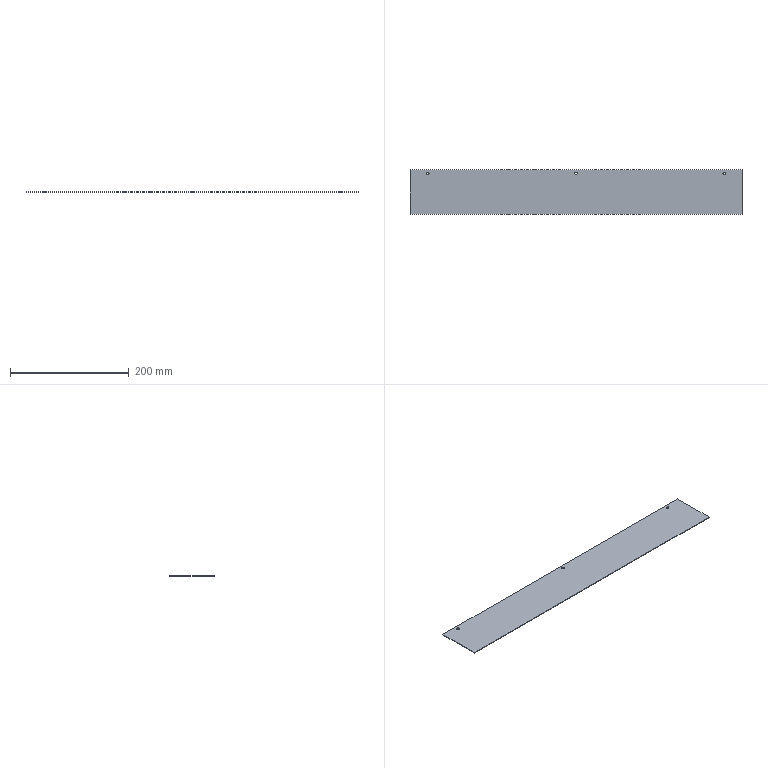Part | SolidWorks | features Cut 1, Extrusion 1 | 1 solid | 12 faces | box 560 x 75 x 1 mm | volume 41952 mm3 | cylinder 6 | plane 6 | commonest cylinder face diameters 4.5 x6
STEP:
#1=CARTESIAN_POINT('',(-2.25,31.5,-0.5));
#2=VERTEX_POINT('',#1);
#3=CARTESIAN_POINT('',(2.25,31.5,-0.5));
#4=VERTEX_POINT('',#3);
#5=CARTESIAN_POINT('',(0.,31.5,-0.5));
#6=DIRECTION('',(0.,0.,1.));
#7=DIRECTION('',(1.,0.,0.));
#8=AXIS2_PLACEMENT_3D('',#5,#6,#7);
#9=CIRCLE('',#8,2.25);
#10=EDGE_CURVE('',#2,#4,#9,.T.);
#11=ORIENTED_EDGE('',*,*,#10,.F.);
#12=CARTESIAN_POINT('',(-2.25,31.5,0.5));
#13=VERTEX_POINT('',#12);
#14=CARTESIAN_POINT('',(-2.25,31.5,-0.5));
#15=DIRECTION('',(0.,0.,1.));
#16=VECTOR('',#15,1000.);
#17=LINE('',#14,#16);
#18=EDGE_CURVE('',#2,#13,#17,.T.);
#19=ORIENTED_EDGE('',*,*,#18,.T.);
#20=CARTESIAN_POINT('',(2.25,31.5,0.5));
#21=VERTEX_POINT('',#20);
#22=CARTESIAN_POINT('',(0.,31.5,0.5));
#23=DIRECTION('',(0.,0.,1.));
#24=DIRECTION('',(1.,0.,0.));
#25=AXIS2_PLACEMENT_3D('',#22,#23,#24);
#26=CIRCLE('',#25,2.25);
#27=EDGE_CURVE('',#13,#21,#26,.T.);
#28=ORIENTED_EDGE('',*,*,#27,.T.);
#29=CARTESIAN_POINT('',(2.25,31.5,-0.5));
#30=DIRECTION('',(0.,0.,1.));
#31=VECTOR('',#30,1000.);
#32=LINE('',#29,#31);
#33=EDGE_CURVE('',#4,#21,#32,.T.);
#34=ORIENTED_EDGE('',*,*,#33,.F.);
#35=EDGE_LOOP('',(#11,#19,#28,#34));
#36=FACE_OUTER_BOUND('',#35,.T.);
#37=CARTESIAN_POINT('',(0.,31.5,-0.5));
#38=DIRECTION('',(0.,0.,1.));
#39=DIRECTION('',(1.,0.,0.));
#40=AXIS2_PLACEMENT_3D('',#37,#38,#39);
#41=CYLINDRICAL_SURFACE('',#40,2.25);
#42=ADVANCED_FACE('',(#36),#41,.F.);
#43=CARTESIAN_POINT('',(247.75,31.5,-0.5));
#44=VERTEX_POINT('',#43);
#45=CARTESIAN_POINT('',(252.25,31.5,-0.5));
#46=VERTEX_POINT('',#45);
#47=CARTESIAN_POINT('',(250.,31.5,-0.5));
#48=DIRECTION('',(0.,0.,1.));
#49=DIRECTION('',(-1.,0.,0.));
#50=AXIS2_PLACEMENT_3D('',#47,#48,#49);
#51=CIRCLE('',#50,2.25);
#52=EDGE_CURVE('',#44,#46,#51,.T.);
#53=ORIENTED_EDGE('',*,*,#52,.F.);
#54=CARTESIAN_POINT('',(247.75,31.5,0.5));
#55=VERTEX_POINT('',#54);
#56=CARTESIAN_POINT('',(247.75,31.5,-0.5));
#57=DIRECTION('',(0.,0.,1.));
#58=VECTOR('',#57,1000.);
#59=LINE('',#56,#58);
#60=EDGE_CURVE('',#44,#55,#59,.T.);
#61=ORIENTED_EDGE('',*,*,#60,.T.);
#62=CARTESIAN_POINT('',(252.25,31.5,0.5));
#63=VERTEX_POINT('',#62);
#64=CARTESIAN_POINT('',(250.,31.5,0.5));
#65=DIRECTION('',(0.,0.,1.));
#66=DIRECTION('',(-1.,0.,0.));
#67=AXIS2_PLACEMENT_3D('',#64,#65,#66);
#68=CIRCLE('',#67,2.25);
#69=EDGE_CURVE('',#55,#63,#68,.T.);
#70=ORIENTED_EDGE('',*,*,#69,.T.);
#71=CARTESIAN_POINT('',(252.25,31.5,-0.5));
#72=DIRECTION('',(0.,0.,1.));
#73=VECTOR('',#72,1000.);
#74=LINE('',#71,#73);
#75=EDGE_CURVE('',#46,#63,#74,.T.);
#76=ORIENTED_EDGE('',*,*,#75,.F.);
#77=EDGE_LOOP('',(#53,#61,#70,#76));
#78=FACE_OUTER_BOUND('',#77,.T.);
#79=CARTESIAN_POINT('',(250.,31.5,-0.5));
#80=DIRECTION('',(0.,0.,1.));
#81=DIRECTION('',(1.,0.,0.));
#82=AXIS2_PLACEMENT_3D('',#79,#80,#81);
#83=CYLINDRICAL_SURFACE('',#82,2.25);
#84=ADVANCED_FACE('',(#78),#83,.F.);
#85=CARTESIAN_POINT('',(-252.25,31.5,-0.5));
#86=VERTEX_POINT('',#85);
#87=CARTESIAN_POINT('',(-247.75,31.5,-0.5));
#88=VERTEX_POINT('',#87);
#89=CARTESIAN_POINT('',(-250.,31.5,-0.5));
#90=DIRECTION('',(0.,0.,1.));
#91=DIRECTION('',(1.,0.,0.));
#92=AXIS2_PLACEMENT_3D('',#89,#90,#91);
#93=CIRCLE('',#92,2.25);
#94=EDGE_CURVE('',#86,#88,#93,.T.);
#95=ORIENTED_EDGE('',*,*,#94,.F.);
#96=CARTESIAN_POINT('',(-252.25,31.5,0.5));
#97=VERTEX_POINT('',#96);
#98=CARTESIAN_POINT('',(-252.25,31.5,-0.5));
#99=DIRECTION('',(0.,0.,1.));
#100=VECTOR('',#99,1000.);
#101=LINE('',#98,#100);
#102=EDGE_CURVE('',#86,#97,#101,.T.);
#103=ORIENTED_EDGE('',*,*,#102,.T.);
#104=CARTESIAN_POINT('',(-247.75,31.5,0.5));
#105=VERTEX_POINT('',#104);
#106=CARTESIAN_POINT('',(-250.,31.5,0.5));
#107=DIRECTION('',(0.,0.,1.));
#108=DIRECTION('',(1.,0.,0.));
#109=AXIS2_PLACEMENT_3D('',#106,#107,#108);
#110=CIRCLE('',#109,2.25);
#111=EDGE_CURVE('',#97,#105,#110,.T.);
#112=ORIENTED_EDGE('',*,*,#111,.T.);
#113=CARTESIAN_POINT('',(-247.75,31.5,-0.5));
#114=DIRECTION('',(0.,0.,1.));
#115=VECTOR('',#114,1000.);
#116=LINE('',#113,#115);
#117=EDGE_CURVE('',#88,#105,#116,.T.);
#118=ORIENTED_EDGE('',*,*,#117,.F.);
#119=EDGE_LOOP('',(#95,#103,#112,#118));
#120=FACE_OUTER_BOUND('',#119,.T.);
#121=CARTESIAN_POINT('',(-250.,31.5,-0.5));
#122=DIRECTION('',(0.,0.,1.));
#123=DIRECTION('',(1.,0.,0.));
#124=AXIS2_PLACEMENT_3D('',#121,#122,#123);
#125=CYLINDRICAL_SURFACE('',#124,2.25);
#126=ADVANCED_FACE('',(#120),#125,.F.);
#127=CARTESIAN_POINT('',(-280.,-37.5,-0.5));
#128=VERTEX_POINT('',#127);
#129=CARTESIAN_POINT('',(-280.,-37.5,0.5));
#130=VERTEX_POINT('',#129);
#131=CARTESIAN_POINT('',(-280.,-37.5,-0.5));
#132=DIRECTION('',(0.,0.,1.));
#133=VECTOR('',#132,1000.);
#134=LINE('',#131,#133);
#135=EDGE_CURVE('',#128,#130,#134,.T.);
#136=ORIENTED_EDGE('',*,*,#135,.T.);
#137=CARTESIAN_POINT('',(-280.,37.5,0.5));
#138=VERTEX_POINT('',#137);
#139=CARTESIAN_POINT('',(-280.,37.5,0.5));
#140=DIRECTION('',(0.,-1.,0.));
#141=VECTOR('',#140,1000.);
#142=LINE('',#139,#141);
#143=EDGE_CURVE('',#138,#130,#142,.T.);
#144=ORIENTED_EDGE('',*,*,#143,.F.);
#145=CARTESIAN_POINT('',(-280.,37.5,-0.5));
#146=VERTEX_POINT('',#145);
#147=CARTESIAN_POINT('',(-280.,37.5,-0.5));
#148=DIRECTION('',(0.,0.,1.));
#149=VECTOR('',#148,1000.);
#150=LINE('',#147,#149);
#151=EDGE_CURVE('',#146,#138,#150,.T.);
#152=ORIENTED_EDGE('',*,*,#151,.F.);
#153=CARTESIAN_POINT('',(-280.,37.5,-0.5));
#154=DIRECTION('',(0.,-1.,0.));
#155=VECTOR('',#154,1000.);
#156=LINE('',#153,#155);
#157=EDGE_CURVE('',#146,#128,#156,.T.);
#158=ORIENTED_EDGE('',*,*,#157,.T.);
#159=EDGE_LOOP('',(#136,#144,#152,#158));
#160=FACE_OUTER_BOUND('',#159,.T.);
#161=CARTESIAN_POINT('',(-280.,37.5,-0.5));
#162=DIRECTION('',(1.,0.,0.));
#163=DIRECTION('',(0.,0.,-1.));
#164=AXIS2_PLACEMENT_3D('',#161,#162,#163);
#165=PLANE('',#164);
#166=ADVANCED_FACE('',(#160),#165,.F.);
#167=CARTESIAN_POINT('',(0.,31.5,0.5));
#168=DIRECTION('',(0.,0.,1.));
#169=DIRECTION('',(1.,0.,0.));
#170=AXIS2_PLACEMENT_3D('',#167,#168,#169);
#171=CIRCLE('',#170,2.25);
#172=EDGE_CURVE('',#21,#13,#171,.T.);
#173=ORIENTED_EDGE('',*,*,#172,.F.);
#174=ORIENTED_EDGE('',*,*,#27,.F.);
#175=EDGE_LOOP('',(#173,#174));
#176=FACE_BOUND('',#175,.T.);
#177=CARTESIAN_POINT('',(250.,31.5,0.5));
#178=DIRECTION('',(0.,0.,1.));
#179=DIRECTION('',(-1.,0.,0.));
#180=AXIS2_PLACEMENT_3D('',#177,#178,#179);
#181=CIRCLE('',#180,2.25);
#182=EDGE_CURVE('',#63,#55,#181,.T.);
#183=ORIENTED_EDGE('',*,*,#182,.F.);
#184=ORIENTED_EDGE('',*,*,#69,.F.);
#185=EDGE_LOOP('',(#183,#184));
#186=FACE_BOUND('',#185,.T.);
#187=CARTESIAN_POINT('',(-250.,31.5,0.5));
#188=DIRECTION('',(0.,0.,1.));
#189=DIRECTION('',(1.,0.,0.));
#190=AXIS2_PLACEMENT_3D('',#187,#188,#189);
#191=CIRCLE('',#190,2.25);
#192=EDGE_CURVE('',#105,#97,#191,.T.);
#193=ORIENTED_EDGE('',*,*,#192,.F.);
#194=ORIENTED_EDGE('',*,*,#111,.F.);
#195=EDGE_LOOP('',(#193,#194));
#196=FACE_BOUND('',#195,.T.);
#197=CARTESIAN_POINT('',(280.,-37.5,0.5));
#198=VERTEX_POINT('',#197);
#199=CARTESIAN_POINT('',(-280.,-37.5,0.5));
#200=DIRECTION('',(1.,0.,0.));
#201=VECTOR('',#200,1000.);
#202=LINE('',#199,#201);
#203=EDGE_CURVE('',#130,#198,#202,.T.);
#204=ORIENTED_EDGE('',*,*,#203,.T.);
#205=CARTESIAN_POINT('',(280.,37.5,0.5));
#206=VERTEX_POINT('',#205);
#207=CARTESIAN_POINT('',(280.,37.5,0.5));
#208=DIRECTION('',(0.,-1.,0.));
#209=VECTOR('',#208,1000.);
#210=LINE('',#207,#209);
#211=EDGE_CURVE('',#206,#198,#210,.T.);
#212=ORIENTED_EDGE('',*,*,#211,.F.);
#213=CARTESIAN_POINT('',(-280.,37.5,0.5));
#214=DIRECTION('',(1.,0.,0.));
#215=VECTOR('',#214,1000.);
#216=LINE('',#213,#215);
#217=EDGE_CURVE('',#138,#206,#216,.T.);
#218=ORIENTED_EDGE('',*,*,#217,.F.);
#219=ORIENTED_EDGE('',*,*,#143,.T.);
#220=EDGE_LOOP('',(#204,#212,#218,#219));
#221=FACE_OUTER_BOUND('',#220,.T.);
#222=CARTESIAN_POINT('',(-280.,37.5,0.5));
#223=DIRECTION('',(0.,0.,-1.));
#224=DIRECTION('',(-1.,0.,0.));
#225=AXIS2_PLACEMENT_3D('',#222,#223,#224);
#226=PLANE('',#225);
#227=ADVANCED_FACE('',(#176,#186,#196,#221),#226,.F.);
#228=CARTESIAN_POINT('',(280.,-37.5,-0.5));
#229=VERTEX_POINT('',#228);
#230=CARTESIAN_POINT('',(280.,-37.5,-0.5));
#231=DIRECTION('',(0.,0.,-1.));
#232=VECTOR('',#231,1000.);
#233=LINE('',#230,#232);
#234=EDGE_CURVE('',#198,#229,#233,.T.);
#235=ORIENTED_EDGE('',*,*,#234,.T.);
#236=CARTESIAN_POINT('',(280.,37.5,-0.5));
#237=VERTEX_POINT('',#236);
#238=CARTESIAN_POINT('',(280.,37.5,-0.5));
#239=DIRECTION('',(0.,-1.,0.));
#240=VECTOR('',#239,1000.);
#241=LINE('',#238,#240);
#242=EDGE_CURVE('',#237,#229,#241,.T.);
#243=ORIENTED_EDGE('',*,*,#242,.F.);
#244=CARTESIAN_POINT('',(280.,37.5,-0.5));
#245=DIRECTION('',(0.,0.,-1.));
#246=VECTOR('',#245,1000.);
#247=LINE('',#244,#246);
#248=EDGE_CURVE('',#206,#237,#247,.T.);
#249=ORIENTED_EDGE('',*,*,#248,.F.);
#250=ORIENTED_EDGE('',*,*,#211,.T.);
#251=EDGE_LOOP('',(#235,#243,#249,#250));
#252=FACE_OUTER_BOUND('',#251,.T.);
#253=CARTESIAN_POINT('',(280.,37.5,-0.5));
#254=DIRECTION('',(-1.,0.,0.));
#255=DIRECTION('',(0.,0.,1.));
#256=AXIS2_PLACEMENT_3D('',#253,#254,#255);
#257=PLANE('',#256);
#258=ADVANCED_FACE('',(#252),#257,.F.);
#259=CARTESIAN_POINT('',(0.,31.5,-0.5));
#260=DIRECTION('',(0.,0.,1.));
#261=DIRECTION('',(1.,0.,0.));
#262=AXIS2_PLACEMENT_3D('',#259,#260,#261);
#263=CIRCLE('',#262,2.25);
#264=EDGE_CURVE('',#4,#2,#263,.T.);
#265=ORIENTED_EDGE('',*,*,#264,.T.);
#266=ORIENTED_EDGE('',*,*,#10,.T.);
#267=EDGE_LOOP('',(#265,#266));
#268=FACE_BOUND('',#267,.T.);
#269=CARTESIAN_POINT('',(250.,31.5,-0.5));
#270=DIRECTION('',(0.,0.,1.));
#271=DIRECTION('',(-1.,0.,0.));
#272=AXIS2_PLACEMENT_3D('',#269,#270,#271);
#273=CIRCLE('',#272,2.25);
#274=EDGE_CURVE('',#46,#44,#273,.T.);
#275=ORIENTED_EDGE('',*,*,#274,.T.);
#276=ORIENTED_EDGE('',*,*,#52,.T.);
#277=EDGE_LOOP('',(#275,#276));
#278=FACE_BOUND('',#277,.T.);
#279=CARTESIAN_POINT('',(-250.,31.5,-0.5));
#280=DIRECTION('',(0.,0.,1.));
#281=DIRECTION('',(1.,0.,0.));
#282=AXIS2_PLACEMENT_3D('',#279,#280,#281);
#283=CIRCLE('',#282,2.25);
#284=EDGE_CURVE('',#88,#86,#283,.T.);
#285=ORIENTED_EDGE('',*,*,#284,.T.);
#286=ORIENTED_EDGE('',*,*,#94,.T.);
#287=EDGE_LOOP('',(#285,#286));
#288=FACE_BOUND('',#287,.T.);
#289=CARTESIAN_POINT('',(-280.,-37.5,-0.5));
#290=DIRECTION('',(-1.,0.,0.));
#291=VECTOR('',#290,1000.);
#292=LINE('',#289,#291);
#293=EDGE_CURVE('',#229,#128,#292,.T.);
#294=ORIENTED_EDGE('',*,*,#293,.T.);
#295=ORIENTED_EDGE('',*,*,#157,.F.);
#296=CARTESIAN_POINT('',(-280.,37.5,-0.5));
#297=DIRECTION('',(-1.,0.,0.));
#298=VECTOR('',#297,1000.);
#299=LINE('',#296,#298);
#300=EDGE_CURVE('',#237,#146,#299,.T.);
#301=ORIENTED_EDGE('',*,*,#300,.F.);
#302=ORIENTED_EDGE('',*,*,#242,.T.);
#303=EDGE_LOOP('',(#294,#295,#301,#302));
#304=FACE_OUTER_BOUND('',#303,.T.);
#305=CARTESIAN_POINT('',(-280.,37.5,-0.5));
#306=DIRECTION('',(0.,0.,1.));
#307=DIRECTION('',(1.,0.,0.));
#308=AXIS2_PLACEMENT_3D('',#305,#306,#307);
#309=PLANE('',#308);
#310=ADVANCED_FACE('',(#268,#278,#288,#304),#309,.F.);
#311=ORIENTED_EDGE('',*,*,#151,.T.);
#312=ORIENTED_EDGE('',*,*,#217,.T.);
#313=ORIENTED_EDGE('',*,*,#248,.T.);
#314=ORIENTED_EDGE('',*,*,#300,.T.);
#315=EDGE_LOOP('',(#311,#312,#313,#314));
#316=FACE_OUTER_BOUND('',#315,.T.);
#317=CARTESIAN_POINT('',(-280.,37.5,0.5));
#318=DIRECTION('',(0.,1.,0.));
#319=DIRECTION('',(0.,0.,1.));
#320=AXIS2_PLACEMENT_3D('',#317,#318,#319);
#321=PLANE('',#320);
#322=ADVANCED_FACE('',(#316),#321,.T.);
#323=ORIENTED_EDGE('',*,*,#135,.F.);
#324=ORIENTED_EDGE('',*,*,#293,.F.);
#325=ORIENTED_EDGE('',*,*,#234,.F.);
#326=ORIENTED_EDGE('',*,*,#203,.F.);
#327=EDGE_LOOP('',(#323,#324,#325,#326));
#328=FACE_OUTER_BOUND('',#327,.T.);
#329=CARTESIAN_POINT('',(-280.,-37.5,0.5));
#330=DIRECTION('',(0.,1.,0.));
#331=DIRECTION('',(0.,0.,1.));
#332=AXIS2_PLACEMENT_3D('',#329,#330,#331);
#333=PLANE('',#332);
#334=ADVANCED_FACE('',(#328),#333,.F.);
#335=ORIENTED_EDGE('',*,*,#102,.F.);
#336=ORIENTED_EDGE('',*,*,#284,.F.);
#337=ORIENTED_EDGE('',*,*,#117,.T.);
#338=ORIENTED_EDGE('',*,*,#192,.T.);
#339=EDGE_LOOP('',(#335,#336,#337,#338));
#340=FACE_OUTER_BOUND('',#339,.T.);
#341=CARTESIAN_POINT('',(-250.,31.5,-0.5));
#342=DIRECTION('',(0.,0.,1.));
#343=DIRECTION('',(1.,0.,0.));
#344=AXIS2_PLACEMENT_3D('',#341,#342,#343);
#345=CYLINDRICAL_SURFACE('',#344,2.25);
#346=ADVANCED_FACE('',(#340),#345,.F.);
#347=ORIENTED_EDGE('',*,*,#60,.F.);
#348=ORIENTED_EDGE('',*,*,#274,.F.);
#349=ORIENTED_EDGE('',*,*,#75,.T.);
#350=ORIENTED_EDGE('',*,*,#182,.T.);
#351=EDGE_LOOP('',(#347,#348,#349,#350));
#352=FACE_OUTER_BOUND('',#351,.T.);
#353=CARTESIAN_POINT('',(250.,31.5,-0.5));
#354=DIRECTION('',(0.,0.,1.));
#355=DIRECTION('',(1.,0.,0.));
#356=AXIS2_PLACEMENT_3D('',#353,#354,#355);
#357=CYLINDRICAL_SURFACE('',#356,2.25);
#358=ADVANCED_FACE('',(#352),#357,.F.);
#359=ORIENTED_EDGE('',*,*,#18,.F.);
#360=ORIENTED_EDGE('',*,*,#264,.F.);
#361=ORIENTED_EDGE('',*,*,#33,.T.);
#362=ORIENTED_EDGE('',*,*,#172,.T.);
#363=EDGE_LOOP('',(#359,#360,#361,#362));
#364=FACE_OUTER_BOUND('',#363,.T.);
#365=CARTESIAN_POINT('',(0.,31.5,-0.5));
#366=DIRECTION('',(0.,0.,1.));
#367=DIRECTION('',(1.,0.,0.));
#368=AXIS2_PLACEMENT_3D('',#365,#366,#367);
#369=CYLINDRICAL_SURFACE('',#368,2.25);
#370=ADVANCED_FACE('',(#364),#369,.F.);
#371=CLOSED_SHELL('',(#42,#84,#126,#166,#227,#258,#310,#322,#334,#346,#358,#370));
#372=MANIFOLD_SOLID_BREP('',#371);
#373=CARTESIAN_POINT('',(0.,0.,0.));
#374=DIRECTION('',(0.,0.,1.));
#375=DIRECTION('',(1.,0.,0.));
#376=AXIS2_PLACEMENT_3D('',#373,#374,#375);
#377=(LENGTH_UNIT()NAMED_UNIT(*)SI_UNIT(.MILLI.,.METRE.));
#378=UNCERTAINTY_MEASURE_WITH_UNIT(LENGTH_MEASURE(0.00001),#377,'','');
#379=(NAMED_UNIT(*)PLANE_ANGLE_UNIT()SI_UNIT($,.RADIAN.));
#380=(NAMED_UNIT(*)SI_UNIT($,.STERADIAN.)SOLID_ANGLE_UNIT());
#381=(GEOMETRIC_REPRESENTATION_CONTEXT(3)GLOBAL_UNCERTAINTY_ASSIGNED_CONTEXT((#378))GLOBAL_UNIT_ASSIGNED_CONTEXT((#377,#379,#380))REPRESENTATION_CONTEXT('',''));
#382=ADVANCED_BREP_SHAPE_REPRESENTATION('',(#372,#376),#381);